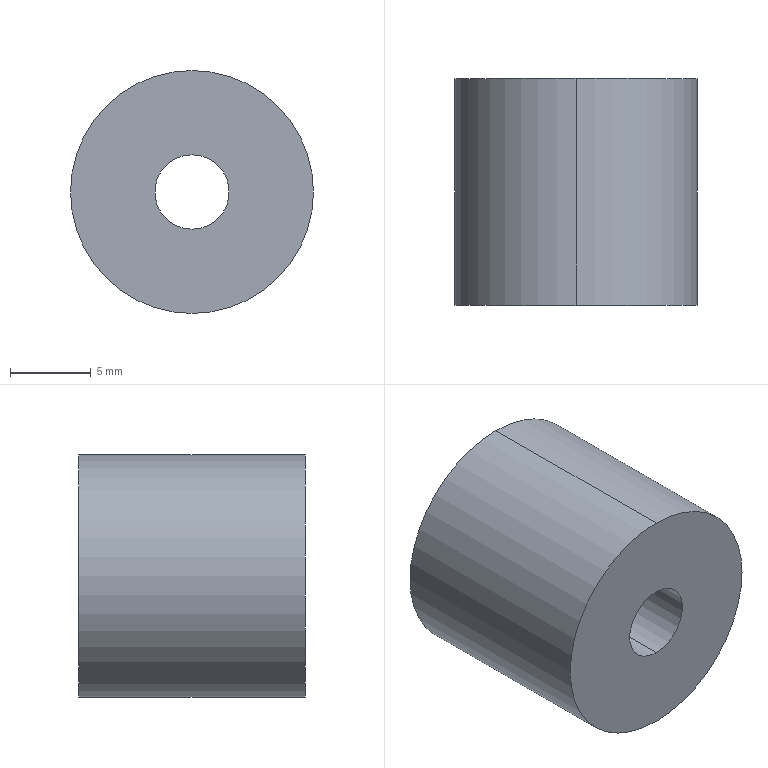Part | STEP file | 1 solid | 9 faces | box 15 x 14 x 15 mm | volume 1932 mm3 | cylinder 6 | plane 3 | commonest cylinder face diameters 4.6 x2 10 x2 15 x2
STEP:
#1=CARTESIAN_POINT('',(0.,0.,0.));
#2=DIRECTION('',(0.,0.,1.));
#3=DIRECTION('',(1.,0.,0.));
#4=AXIS2_PLACEMENT_3D('',#1,#2,#3);
#5=CARTESIAN_POINT('',(0.,14.,7.5));
#6=VERTEX_POINT('',#5);
#7=CARTESIAN_POINT('',(0.,0.,7.5));
#8=VERTEX_POINT('',#7);
#9=CARTESIAN_POINT('',(0.,0.,7.5));
#10=DIRECTION('',(0.,-1.,0.));
#11=VECTOR('',#10,1.);
#12=LINE('',#9,#11);
#13=CARTESIAN_POINT('',(0.,0.,0.));
#14=DIRECTION('',(0.,-1.,0.));
#15=DIRECTION('',(0.,0.,-1.));
#16=AXIS2_PLACEMENT_3D('',#13,#14,#15);
#17=CYLINDRICAL_SURFACE('',#16,7.5);
#18=CARTESIAN_POINT('',(3.142,0.));
#19=DIRECTION('',(0.,1.));
#20=VECTOR('',#19,1.);
#21=LINE('',#18,#20);
#22=(GEOMETRIC_REPRESENTATION_CONTEXT(2)PARAMETRIC_REPRESENTATION_CONTEXT()REPRESENTATION_CONTEXT('',''));
#23=DEFINITIONAL_REPRESENTATION('',(#21),#22);
#24=PCURVE('',#17,#23);
#25=CARTESIAN_POINT('',(0.,0.,0.));
#26=DIRECTION('',(0.,-1.,0.));
#27=DIRECTION('',(0.,0.,-1.));
#28=AXIS2_PLACEMENT_3D('',#25,#26,#27);
#29=CYLINDRICAL_SURFACE('',#28,7.5);
#30=CARTESIAN_POINT('',(3.142,0.));
#31=DIRECTION('',(0.,1.));
#32=VECTOR('',#31,1.);
#33=LINE('',#30,#32);
#34=(GEOMETRIC_REPRESENTATION_CONTEXT(2)PARAMETRIC_REPRESENTATION_CONTEXT()REPRESENTATION_CONTEXT('',''));
#35=DEFINITIONAL_REPRESENTATION('',(#33),#34);
#36=PCURVE('',#29,#35);
#37=SURFACE_CURVE('',#12,(#24,#36),.PCURVE_S1.);
#38=EDGE_CURVE('',#6,#8,#37,.T.);
#39=ORIENTED_EDGE('',*,*,#38,.F.);
#40=CARTESIAN_POINT('',(0.,14.,-7.5));
#41=VERTEX_POINT('',#40);
#42=CARTESIAN_POINT('',(0.,14.,0.));
#43=DIRECTION('',(0.,-1.,0.));
#44=DIRECTION('',(0.,0.,-1.));
#45=AXIS2_PLACEMENT_3D('',#42,#43,#44);
#46=CIRCLE('',#45,7.5);
#47=CARTESIAN_POINT('',(0.,-14.));
#48=DIRECTION('',(1.,0.));
#49=VECTOR('',#48,1.);
#50=LINE('',#47,#49);
#51=(GEOMETRIC_REPRESENTATION_CONTEXT(2)PARAMETRIC_REPRESENTATION_CONTEXT()REPRESENTATION_CONTEXT('',''));
#52=DEFINITIONAL_REPRESENTATION('',(#50),#51);
#53=PCURVE('',#17,#52);
#54=CARTESIAN_POINT('',(-5.,14.,0.));
#55=DIRECTION('',(0.,-1.,0.));
#56=DIRECTION('',(0.,0.,-1.));
#57=AXIS2_PLACEMENT_3D('',#54,#55,#56);
#58=PLANE('',#57);
#59=CARTESIAN_POINT('',(0.,5.));
#60=DIRECTION('',(1.,0.));
#61=AXIS2_PLACEMENT_2D('',#59,#60);
#62=CIRCLE('',#61,7.5);
#63=(GEOMETRIC_REPRESENTATION_CONTEXT(2)PARAMETRIC_REPRESENTATION_CONTEXT()REPRESENTATION_CONTEXT('',''));
#64=DEFINITIONAL_REPRESENTATION('',(#62),#63);
#65=PCURVE('',#58,#64);
#66=SURFACE_CURVE('',#46,(#53,#65),.PCURVE_S1.);
#67=EDGE_CURVE('',#6,#41,#66,.T.);
#68=ORIENTED_EDGE('',*,*,#67,.T.);
#69=CARTESIAN_POINT('',(0.,0.,-7.5));
#70=VERTEX_POINT('',#69);
#71=CARTESIAN_POINT('',(0.,0.,-7.5));
#72=DIRECTION('',(0.,-1.,0.));
#73=VECTOR('',#72,1.);
#74=LINE('',#71,#73);
#75=CARTESIAN_POINT('',(6.283,0.));
#76=DIRECTION('',(0.,1.));
#77=VECTOR('',#76,1.);
#78=LINE('',#75,#77);
#79=(GEOMETRIC_REPRESENTATION_CONTEXT(2)PARAMETRIC_REPRESENTATION_CONTEXT()REPRESENTATION_CONTEXT('',''));
#80=DEFINITIONAL_REPRESENTATION('',(#78),#79);
#81=PCURVE('',#17,#80);
#82=CARTESIAN_POINT('',(0.,0.));
#83=DIRECTION('',(0.,1.));
#84=VECTOR('',#83,1.);
#85=LINE('',#82,#84);
#86=(GEOMETRIC_REPRESENTATION_CONTEXT(2)PARAMETRIC_REPRESENTATION_CONTEXT()REPRESENTATION_CONTEXT('',''));
#87=DEFINITIONAL_REPRESENTATION('',(#85),#86);
#88=PCURVE('',#29,#87);
#89=SURFACE_CURVE('',#74,(#81,#88),.PCURVE_S1.);
#90=EDGE_CURVE('',#41,#70,#89,.T.);
#91=ORIENTED_EDGE('',*,*,#90,.T.);
#92=CARTESIAN_POINT('',(0.,0.,0.));
#93=DIRECTION('',(0.,-1.,0.));
#94=DIRECTION('',(0.,0.,-1.));
#95=AXIS2_PLACEMENT_3D('',#92,#93,#94);
#96=CIRCLE('',#95,7.5);
#97=CARTESIAN_POINT('',(0.,0.));
#98=DIRECTION('',(1.,0.));
#99=VECTOR('',#98,1.);
#100=LINE('',#97,#99);
#101=(GEOMETRIC_REPRESENTATION_CONTEXT(2)PARAMETRIC_REPRESENTATION_CONTEXT()REPRESENTATION_CONTEXT('',''));
#102=DEFINITIONAL_REPRESENTATION('',(#100),#101);
#103=PCURVE('',#17,#102);
#104=CARTESIAN_POINT('',(-7.5,0.,0.));
#105=DIRECTION('',(0.,1.,0.));
#106=DIRECTION('',(0.,0.,1.));
#107=AXIS2_PLACEMENT_3D('',#104,#105,#106);
#108=PLANE('',#107);
#109=CARTESIAN_POINT('',(-7.5,7.5));
#110=CARTESIAN_POINT('',(-7.5,20.49));
#111=CARTESIAN_POINT('',(3.75,13.995));
#112=CARTESIAN_POINT('',(15.,7.5));
#113=CARTESIAN_POINT('',(3.75,1.005));
#114=CARTESIAN_POINT('',(-7.5,-5.49));
#115=CARTESIAN_POINT('',(-7.5,7.5));
#116=(BOUNDED_CURVE()B_SPLINE_CURVE(2,(#109,#110,#111,#112,#113,#114,#115),.UNSPECIFIED.,.T.,.F.)B_SPLINE_CURVE_WITH_KNOTS((1,2,2,2,2,1),(-2.094,0.,2.094,4.189,6.283,8.378),.UNSPECIFIED.)CURVE()GEOMETRIC_REPRESENTATION_ITEM()RATIONAL_B_SPLINE_CURVE((1.,0.5,1.,0.5,1.,0.5,1.))REPRESENTATION_ITEM(''));
#117=(GEOMETRIC_REPRESENTATION_CONTEXT(2)PARAMETRIC_REPRESENTATION_CONTEXT()REPRESENTATION_CONTEXT('',''));
#118=DEFINITIONAL_REPRESENTATION('',(#116),#117);
#119=PCURVE('',#108,#118);
#120=SURFACE_CURVE('',#96,(#103,#119),.PCURVE_S1.);
#121=EDGE_CURVE('',#8,#70,#120,.T.);
#122=ORIENTED_EDGE('',*,*,#121,.F.);
#123=EDGE_LOOP('',(#39,#68,#91,#122));
#124=FACE_BOUND('',#123,.T.);
#125=ADVANCED_FACE('',(#124),#17,.T.);
#126=CARTESIAN_POINT('',(0.,14.,-5.));
#127=VERTEX_POINT('',#126);
#128=CARTESIAN_POINT('',(0.,14.,5.));
#129=VERTEX_POINT('',#128);
#130=CARTESIAN_POINT('',(0.,14.,0.));
#131=DIRECTION('',(0.,-1.,0.));
#132=DIRECTION('',(0.,0.,-1.));
#133=AXIS2_PLACEMENT_3D('',#130,#131,#132);
#134=CIRCLE('',#133,5.);
#135=CARTESIAN_POINT('',(0.,5.));
#136=DIRECTION('',(1.,0.));
#137=AXIS2_PLACEMENT_2D('',#135,#136);
#138=CIRCLE('',#137,5.);
#139=(GEOMETRIC_REPRESENTATION_CONTEXT(2)PARAMETRIC_REPRESENTATION_CONTEXT()REPRESENTATION_CONTEXT('',''));
#140=DEFINITIONAL_REPRESENTATION('',(#138),#139);
#141=PCURVE('',#58,#140);
#142=CARTESIAN_POINT('',(0.,0.,0.));
#143=DIRECTION('',(0.,-1.,0.));
#144=DIRECTION('',(0.,0.,-1.));
#145=AXIS2_PLACEMENT_3D('',#142,#143,#144);
#146=CYLINDRICAL_SURFACE('',#145,5.);
#147=CARTESIAN_POINT('',(0.,-14.));
#148=DIRECTION('',(1.,0.));
#149=VECTOR('',#148,1.);
#150=LINE('',#147,#149);
#151=(GEOMETRIC_REPRESENTATION_CONTEXT(2)PARAMETRIC_REPRESENTATION_CONTEXT()REPRESENTATION_CONTEXT('',''));
#152=DEFINITIONAL_REPRESENTATION('',(#150),#151);
#153=PCURVE('',#146,#152);
#154=SURFACE_CURVE('',#134,(#141,#153),.PCURVE_S1.);
#155=EDGE_CURVE('',#127,#129,#154,.T.);
#156=ORIENTED_EDGE('',*,*,#155,.T.);
#157=CARTESIAN_POINT('',(0.,14.,0.));
#158=DIRECTION('',(0.,-1.,0.));
#159=DIRECTION('',(0.,0.,-1.));
#160=AXIS2_PLACEMENT_3D('',#157,#158,#159);
#161=CIRCLE('',#160,5.);
#162=CARTESIAN_POINT('',(0.,5.));
#163=DIRECTION('',(1.,0.));
#164=AXIS2_PLACEMENT_2D('',#162,#163);
#165=CIRCLE('',#164,5.);
#166=(GEOMETRIC_REPRESENTATION_CONTEXT(2)PARAMETRIC_REPRESENTATION_CONTEXT()REPRESENTATION_CONTEXT('',''));
#167=DEFINITIONAL_REPRESENTATION('',(#165),#166);
#168=PCURVE('',#58,#167);
#169=CARTESIAN_POINT('',(0.,0.,0.));
#170=DIRECTION('',(0.,-1.,0.));
#171=DIRECTION('',(0.,0.,-1.));
#172=AXIS2_PLACEMENT_3D('',#169,#170,#171);
#173=CYLINDRICAL_SURFACE('',#172,5.);
#174=CARTESIAN_POINT('',(0.,-14.));
#175=DIRECTION('',(1.,0.));
#176=VECTOR('',#175,1.);
#177=LINE('',#174,#176);
#178=(GEOMETRIC_REPRESENTATION_CONTEXT(2)PARAMETRIC_REPRESENTATION_CONTEXT()REPRESENTATION_CONTEXT('',''));
#179=DEFINITIONAL_REPRESENTATION('',(#177),#178);
#180=PCURVE('',#173,#179);
#181=SURFACE_CURVE('',#161,(#168,#180),.PCURVE_S1.);
#182=EDGE_CURVE('',#129,#127,#181,.T.);
#183=ORIENTED_EDGE('',*,*,#182,.T.);
#184=EDGE_LOOP('',(#156,#183));
#185=FACE_BOUND('',#184,.T.);
#186=CARTESIAN_POINT('',(0.,14.,0.));
#187=DIRECTION('',(0.,-1.,0.));
#188=DIRECTION('',(0.,0.,-1.));
#189=AXIS2_PLACEMENT_3D('',#186,#187,#188);
#190=CIRCLE('',#189,7.5);
#191=CARTESIAN_POINT('',(0.,5.));
#192=DIRECTION('',(1.,0.));
#193=AXIS2_PLACEMENT_2D('',#191,#192);
#194=CIRCLE('',#193,7.5);
#195=(GEOMETRIC_REPRESENTATION_CONTEXT(2)PARAMETRIC_REPRESENTATION_CONTEXT()REPRESENTATION_CONTEXT('',''));
#196=DEFINITIONAL_REPRESENTATION('',(#194),#195);
#197=PCURVE('',#58,#196);
#198=CARTESIAN_POINT('',(0.,-14.));
#199=DIRECTION('',(1.,0.));
#200=VECTOR('',#199,1.);
#201=LINE('',#198,#200);
#202=(GEOMETRIC_REPRESENTATION_CONTEXT(2)PARAMETRIC_REPRESENTATION_CONTEXT()REPRESENTATION_CONTEXT('',''));
#203=DEFINITIONAL_REPRESENTATION('',(#201),#202);
#204=PCURVE('',#29,#203);
#205=SURFACE_CURVE('',#190,(#197,#204),.PCURVE_S1.);
#206=EDGE_CURVE('',#41,#6,#205,.T.);
#207=ORIENTED_EDGE('',*,*,#206,.F.);
#208=ORIENTED_EDGE('',*,*,#67,.F.);
#209=EDGE_LOOP('',(#207,#208));
#210=FACE_BOUND('',#209,.T.);
#211=ADVANCED_FACE('',(#185,#210),#58,.F.);
#212=CARTESIAN_POINT('',(0.,9.,-5.));
#213=VERTEX_POINT('',#212);
#214=CARTESIAN_POINT('',(0.,9.,5.));
#215=VERTEX_POINT('',#214);
#216=CARTESIAN_POINT('',(0.,9.,0.));
#217=DIRECTION('',(0.,-1.,0.));
#218=DIRECTION('',(0.,0.,-1.));
#219=AXIS2_PLACEMENT_3D('',#216,#217,#218);
#220=CIRCLE('',#219,5.);
#221=CARTESIAN_POINT('',(0.,-9.));
#222=DIRECTION('',(1.,0.));
#223=VECTOR('',#222,1.);
#224=LINE('',#221,#223);
#225=(GEOMETRIC_REPRESENTATION_CONTEXT(2)PARAMETRIC_REPRESENTATION_CONTEXT()REPRESENTATION_CONTEXT('',''));
#226=DEFINITIONAL_REPRESENTATION('',(#224),#225);
#227=PCURVE('',#146,#226);
#228=CARTESIAN_POINT('',(-2.3,9.,0.));
#229=DIRECTION('',(0.,-1.,0.));
#230=DIRECTION('',(0.,0.,-1.));
#231=AXIS2_PLACEMENT_3D('',#228,#229,#230);
#232=PLANE('',#231);
#233=CARTESIAN_POINT('',(0.,2.3));
#234=DIRECTION('',(1.,0.));
#235=AXIS2_PLACEMENT_2D('',#233,#234);
#236=CIRCLE('',#235,5.);
#237=(GEOMETRIC_REPRESENTATION_CONTEXT(2)PARAMETRIC_REPRESENTATION_CONTEXT()REPRESENTATION_CONTEXT('',''));
#238=DEFINITIONAL_REPRESENTATION('',(#236),#237);
#239=PCURVE('',#232,#238);
#240=SURFACE_CURVE('',#220,(#227,#239),.PCURVE_S1.);
#241=EDGE_CURVE('',#213,#215,#240,.T.);
#242=ORIENTED_EDGE('',*,*,#241,.F.);
#243=CARTESIAN_POINT('',(0.,0.,-5.));
#244=DIRECTION('',(0.,-1.,0.));
#245=VECTOR('',#244,1.);
#246=LINE('',#243,#245);
#247=CARTESIAN_POINT('',(0.,0.));
#248=DIRECTION('',(0.,1.));
#249=VECTOR('',#248,1.);
#250=LINE('',#247,#249);
#251=(GEOMETRIC_REPRESENTATION_CONTEXT(2)PARAMETRIC_REPRESENTATION_CONTEXT()REPRESENTATION_CONTEXT('',''));
#252=DEFINITIONAL_REPRESENTATION('',(#250),#251);
#253=PCURVE('',#146,#252);
#254=CARTESIAN_POINT('',(6.283,0.));
#255=DIRECTION('',(0.,1.));
#256=VECTOR('',#255,1.);
#257=LINE('',#254,#256);
#258=(GEOMETRIC_REPRESENTATION_CONTEXT(2)PARAMETRIC_REPRESENTATION_CONTEXT()REPRESENTATION_CONTEXT('',''));
#259=DEFINITIONAL_REPRESENTATION('',(#257),#258);
#260=PCURVE('',#173,#259);
#261=SURFACE_CURVE('',#246,(#253,#260),.PCURVE_S1.);
#262=EDGE_CURVE('',#127,#213,#261,.T.);
#263=ORIENTED_EDGE('',*,*,#262,.F.);
#264=ORIENTED_EDGE('',*,*,#155,.T.);
#265=CARTESIAN_POINT('',(0.,0.,5.));
#266=DIRECTION('',(0.,-1.,0.));
#267=VECTOR('',#266,1.);
#268=LINE('',#265,#267);
#269=CARTESIAN_POINT('',(3.142,0.));
#270=DIRECTION('',(0.,1.));
#271=VECTOR('',#270,1.);
#272=LINE('',#269,#271);
#273=(GEOMETRIC_REPRESENTATION_CONTEXT(2)PARAMETRIC_REPRESENTATION_CONTEXT()REPRESENTATION_CONTEXT('',''));
#274=DEFINITIONAL_REPRESENTATION('',(#272),#273);
#275=PCURVE('',#146,#274);
#276=CARTESIAN_POINT('',(3.142,0.));
#277=DIRECTION('',(0.,1.));
#278=VECTOR('',#277,1.);
#279=LINE('',#276,#278);
#280=(GEOMETRIC_REPRESENTATION_CONTEXT(2)PARAMETRIC_REPRESENTATION_CONTEXT()REPRESENTATION_CONTEXT('',''));
#281=DEFINITIONAL_REPRESENTATION('',(#279),#280);
#282=PCURVE('',#173,#281);
#283=SURFACE_CURVE('',#268,(#275,#282),.PCURVE_S1.);
#284=EDGE_CURVE('',#129,#215,#283,.T.);
#285=ORIENTED_EDGE('',*,*,#284,.T.);
#286=EDGE_LOOP('',(#242,#263,#264,#285));
#287=FACE_BOUND('',#286,.F.);
#288=ADVANCED_FACE('',(#287),#146,.F.);
#289=CARTESIAN_POINT('',(0.,9.,-2.3));
#290=VERTEX_POINT('',#289);
#291=CARTESIAN_POINT('',(0.,9.,2.3));
#292=VERTEX_POINT('',#291);
#293=CARTESIAN_POINT('',(0.,9.,0.));
#294=DIRECTION('',(0.,-1.,0.));
#295=DIRECTION('',(0.,0.,-1.));
#296=AXIS2_PLACEMENT_3D('',#293,#294,#295);
#297=CIRCLE('',#296,2.3);
#298=CARTESIAN_POINT('',(0.,2.3));
#299=DIRECTION('',(1.,0.));
#300=AXIS2_PLACEMENT_2D('',#298,#299);
#301=CIRCLE('',#300,2.3);
#302=(GEOMETRIC_REPRESENTATION_CONTEXT(2)PARAMETRIC_REPRESENTATION_CONTEXT()REPRESENTATION_CONTEXT('',''));
#303=DEFINITIONAL_REPRESENTATION('',(#301),#302);
#304=PCURVE('',#232,#303);
#305=CARTESIAN_POINT('',(0.,0.,0.));
#306=DIRECTION('',(0.,-1.,0.));
#307=DIRECTION('',(0.,0.,-1.));
#308=AXIS2_PLACEMENT_3D('',#305,#306,#307);
#309=CYLINDRICAL_SURFACE('',#308,2.3);
#310=CARTESIAN_POINT('',(0.,-9.));
#311=DIRECTION('',(1.,0.));
#312=VECTOR('',#311,1.);
#313=LINE('',#310,#312);
#314=(GEOMETRIC_REPRESENTATION_CONTEXT(2)PARAMETRIC_REPRESENTATION_CONTEXT()REPRESENTATION_CONTEXT('',''));
#315=DEFINITIONAL_REPRESENTATION('',(#313),#314);
#316=PCURVE('',#309,#315);
#317=SURFACE_CURVE('',#297,(#304,#316),.PCURVE_S1.);
#318=EDGE_CURVE('',#290,#292,#317,.T.);
#319=ORIENTED_EDGE('',*,*,#318,.T.);
#320=CARTESIAN_POINT('',(0.,9.,0.));
#321=DIRECTION('',(0.,-1.,0.));
#322=DIRECTION('',(0.,0.,-1.));
#323=AXIS2_PLACEMENT_3D('',#320,#321,#322);
#324=CIRCLE('',#323,2.3);
#325=CARTESIAN_POINT('',(0.,2.3));
#326=DIRECTION('',(1.,0.));
#327=AXIS2_PLACEMENT_2D('',#325,#326);
#328=CIRCLE('',#327,2.3);
#329=(GEOMETRIC_REPRESENTATION_CONTEXT(2)PARAMETRIC_REPRESENTATION_CONTEXT()REPRESENTATION_CONTEXT('',''));
#330=DEFINITIONAL_REPRESENTATION('',(#328),#329);
#331=PCURVE('',#232,#330);
#332=CARTESIAN_POINT('',(0.,0.,0.));
#333=DIRECTION('',(0.,-1.,0.));
#334=DIRECTION('',(0.,0.,-1.));
#335=AXIS2_PLACEMENT_3D('',#332,#333,#334);
#336=CYLINDRICAL_SURFACE('',#335,2.3);
#337=CARTESIAN_POINT('',(0.,-9.));
#338=DIRECTION('',(1.,0.));
#339=VECTOR('',#338,1.);
#340=LINE('',#337,#339);
#341=(GEOMETRIC_REPRESENTATION_CONTEXT(2)PARAMETRIC_REPRESENTATION_CONTEXT()REPRESENTATION_CONTEXT('',''));
#342=DEFINITIONAL_REPRESENTATION('',(#340),#341);
#343=PCURVE('',#336,#342);
#344=SURFACE_CURVE('',#324,(#331,#343),.PCURVE_S1.);
#345=EDGE_CURVE('',#292,#290,#344,.T.);
#346=ORIENTED_EDGE('',*,*,#345,.T.);
#347=EDGE_LOOP('',(#319,#346));
#348=FACE_BOUND('',#347,.T.);
#349=ORIENTED_EDGE('',*,*,#241,.F.);
#350=CARTESIAN_POINT('',(0.,9.,0.));
#351=DIRECTION('',(0.,-1.,0.));
#352=DIRECTION('',(0.,0.,-1.));
#353=AXIS2_PLACEMENT_3D('',#350,#351,#352);
#354=CIRCLE('',#353,5.);
#355=CARTESIAN_POINT('',(0.,2.3));
#356=DIRECTION('',(1.,0.));
#357=AXIS2_PLACEMENT_2D('',#355,#356);
#358=CIRCLE('',#357,5.);
#359=(GEOMETRIC_REPRESENTATION_CONTEXT(2)PARAMETRIC_REPRESENTATION_CONTEXT()REPRESENTATION_CONTEXT('',''));
#360=DEFINITIONAL_REPRESENTATION('',(#358),#359);
#361=PCURVE('',#232,#360);
#362=CARTESIAN_POINT('',(0.,-9.));
#363=DIRECTION('',(1.,0.));
#364=VECTOR('',#363,1.);
#365=LINE('',#362,#364);
#366=(GEOMETRIC_REPRESENTATION_CONTEXT(2)PARAMETRIC_REPRESENTATION_CONTEXT()REPRESENTATION_CONTEXT('',''));
#367=DEFINITIONAL_REPRESENTATION('',(#365),#366);
#368=PCURVE('',#173,#367);
#369=SURFACE_CURVE('',#354,(#361,#368),.PCURVE_S1.);
#370=EDGE_CURVE('',#215,#213,#369,.T.);
#371=ORIENTED_EDGE('',*,*,#370,.F.);
#372=EDGE_LOOP('',(#349,#371));
#373=FACE_BOUND('',#372,.T.);
#374=ADVANCED_FACE('',(#348,#373),#232,.F.);
#375=CARTESIAN_POINT('',(0.,0.,-2.3));
#376=VERTEX_POINT('',#375);
#377=CARTESIAN_POINT('',(0.,0.,2.3));
#378=VERTEX_POINT('',#377);
#379=CARTESIAN_POINT('',(0.,0.,0.));
#380=DIRECTION('',(0.,-1.,0.));
#381=DIRECTION('',(0.,0.,-1.));
#382=AXIS2_PLACEMENT_3D('',#379,#380,#381);
#383=CIRCLE('',#382,2.3);
#384=CARTESIAN_POINT('',(0.,0.));
#385=DIRECTION('',(1.,0.));
#386=VECTOR('',#385,1.);
#387=LINE('',#384,#386);
#388=(GEOMETRIC_REPRESENTATION_CONTEXT(2)PARAMETRIC_REPRESENTATION_CONTEXT()REPRESENTATION_CONTEXT('',''));
#389=DEFINITIONAL_REPRESENTATION('',(#387),#388);
#390=PCURVE('',#309,#389);
#391=CARTESIAN_POINT('',(-2.3,7.5));
#392=CARTESIAN_POINT('',(-2.3,11.484));
#393=CARTESIAN_POINT('',(1.15,9.492));
#394=CARTESIAN_POINT('',(4.6,7.5));
#395=CARTESIAN_POINT('',(1.15,5.508));
#396=CARTESIAN_POINT('',(-2.3,3.516));
#397=CARTESIAN_POINT('',(-2.3,7.5));
#398=(BOUNDED_CURVE()B_SPLINE_CURVE(2,(#391,#392,#393,#394,#395,#396,#397),.UNSPECIFIED.,.T.,.F.)B_SPLINE_CURVE_WITH_KNOTS((1,2,2,2,2,1),(-2.094,0.,2.094,4.189,6.283,8.378),.UNSPECIFIED.)CURVE()GEOMETRIC_REPRESENTATION_ITEM()RATIONAL_B_SPLINE_CURVE((1.,0.5,1.,0.5,1.,0.5,1.))REPRESENTATION_ITEM(''));
#399=(GEOMETRIC_REPRESENTATION_CONTEXT(2)PARAMETRIC_REPRESENTATION_CONTEXT()REPRESENTATION_CONTEXT('',''));
#400=DEFINITIONAL_REPRESENTATION('',(#398),#399);
#401=PCURVE('',#108,#400);
#402=SURFACE_CURVE('',#383,(#390,#401),.PCURVE_S1.);
#403=EDGE_CURVE('',#376,#378,#402,.T.);
#404=ORIENTED_EDGE('',*,*,#403,.F.);
#405=CARTESIAN_POINT('',(0.,0.,-2.3));
#406=DIRECTION('',(0.,-1.,0.));
#407=VECTOR('',#406,1.);
#408=LINE('',#405,#407);
#409=CARTESIAN_POINT('',(0.,0.));
#410=DIRECTION('',(0.,1.));
#411=VECTOR('',#410,1.);
#412=LINE('',#409,#411);
#413=(GEOMETRIC_REPRESENTATION_CONTEXT(2)PARAMETRIC_REPRESENTATION_CONTEXT()REPRESENTATION_CONTEXT('',''));
#414=DEFINITIONAL_REPRESENTATION('',(#412),#413);
#415=PCURVE('',#309,#414);
#416=CARTESIAN_POINT('',(6.283,0.));
#417=DIRECTION('',(0.,1.));
#418=VECTOR('',#417,1.);
#419=LINE('',#416,#418);
#420=(GEOMETRIC_REPRESENTATION_CONTEXT(2)PARAMETRIC_REPRESENTATION_CONTEXT()REPRESENTATION_CONTEXT('',''));
#421=DEFINITIONAL_REPRESENTATION('',(#419),#420);
#422=PCURVE('',#336,#421);
#423=SURFACE_CURVE('',#408,(#415,#422),.PCURVE_S1.);
#424=EDGE_CURVE('',#290,#376,#423,.T.);
#425=ORIENTED_EDGE('',*,*,#424,.F.);
#426=ORIENTED_EDGE('',*,*,#318,.T.);
#427=CARTESIAN_POINT('',(0.,0.,2.3));
#428=DIRECTION('',(0.,-1.,0.));
#429=VECTOR('',#428,1.);
#430=LINE('',#427,#429);
#431=CARTESIAN_POINT('',(3.142,0.));
#432=DIRECTION('',(0.,1.));
#433=VECTOR('',#432,1.);
#434=LINE('',#431,#433);
#435=(GEOMETRIC_REPRESENTATION_CONTEXT(2)PARAMETRIC_REPRESENTATION_CONTEXT()REPRESENTATION_CONTEXT('',''));
#436=DEFINITIONAL_REPRESENTATION('',(#434),#435);
#437=PCURVE('',#309,#436);
#438=CARTESIAN_POINT('',(3.142,0.));
#439=DIRECTION('',(0.,1.));
#440=VECTOR('',#439,1.);
#441=LINE('',#438,#440);
#442=(GEOMETRIC_REPRESENTATION_CONTEXT(2)PARAMETRIC_REPRESENTATION_CONTEXT()REPRESENTATION_CONTEXT('',''));
#443=DEFINITIONAL_REPRESENTATION('',(#441),#442);
#444=PCURVE('',#336,#443);
#445=SURFACE_CURVE('',#430,(#437,#444),.PCURVE_S1.);
#446=EDGE_CURVE('',#292,#378,#445,.T.);
#447=ORIENTED_EDGE('',*,*,#446,.T.);
#448=EDGE_LOOP('',(#404,#425,#426,#447));
#449=FACE_BOUND('',#448,.F.);
#450=ADVANCED_FACE('',(#449),#309,.F.);
#451=CARTESIAN_POINT('',(0.,0.,0.));
#452=DIRECTION('',(0.,-1.,0.));
#453=DIRECTION('',(0.,0.,-1.));
#454=AXIS2_PLACEMENT_3D('',#451,#452,#453);
#455=CIRCLE('',#454,7.5);
#456=CARTESIAN_POINT('',(-7.5,7.5));
#457=CARTESIAN_POINT('',(-7.5,20.49));
#458=CARTESIAN_POINT('',(3.75,13.995));
#459=CARTESIAN_POINT('',(15.,7.5));
#460=CARTESIAN_POINT('',(3.75,1.005));
#461=CARTESIAN_POINT('',(-7.5,-5.49));
#462=CARTESIAN_POINT('',(-7.5,7.5));
#463=(BOUNDED_CURVE()B_SPLINE_CURVE(2,(#456,#457,#458,#459,#460,#461,#462),.UNSPECIFIED.,.T.,.F.)B_SPLINE_CURVE_WITH_KNOTS((1,2,2,2,2,1),(-2.094,0.,2.094,4.189,6.283,8.378),.UNSPECIFIED.)CURVE()GEOMETRIC_REPRESENTATION_ITEM()RATIONAL_B_SPLINE_CURVE((1.,0.5,1.,0.5,1.,0.5,1.))REPRESENTATION_ITEM(''));
#464=(GEOMETRIC_REPRESENTATION_CONTEXT(2)PARAMETRIC_REPRESENTATION_CONTEXT()REPRESENTATION_CONTEXT('',''));
#465=DEFINITIONAL_REPRESENTATION('',(#463),#464);
#466=PCURVE('',#108,#465);
#467=CARTESIAN_POINT('',(0.,0.));
#468=DIRECTION('',(1.,0.));
#469=VECTOR('',#468,1.);
#470=LINE('',#467,#469);
#471=(GEOMETRIC_REPRESENTATION_CONTEXT(2)PARAMETRIC_REPRESENTATION_CONTEXT()REPRESENTATION_CONTEXT('',''));
#472=DEFINITIONAL_REPRESENTATION('',(#470),#471);
#473=PCURVE('',#29,#472);
#474=SURFACE_CURVE('',#455,(#466,#473),.PCURVE_S1.);
#475=EDGE_CURVE('',#70,#8,#474,.T.);
#476=ORIENTED_EDGE('',*,*,#475,.T.);
#477=ORIENTED_EDGE('',*,*,#121,.T.);
#478=EDGE_LOOP('',(#476,#477));
#479=FACE_BOUND('',#478,.T.);
#480=ORIENTED_EDGE('',*,*,#403,.F.);
#481=CARTESIAN_POINT('',(0.,0.,0.));
#482=DIRECTION('',(0.,-1.,0.));
#483=DIRECTION('',(0.,0.,-1.));
#484=AXIS2_PLACEMENT_3D('',#481,#482,#483);
#485=CIRCLE('',#484,2.3);
#486=CARTESIAN_POINT('',(-2.3,7.5));
#487=CARTESIAN_POINT('',(-2.3,11.484));
#488=CARTESIAN_POINT('',(1.15,9.492));
#489=CARTESIAN_POINT('',(4.6,7.5));
#490=CARTESIAN_POINT('',(1.15,5.508));
#491=CARTESIAN_POINT('',(-2.3,3.516));
#492=CARTESIAN_POINT('',(-2.3,7.5));
#493=(BOUNDED_CURVE()B_SPLINE_CURVE(2,(#486,#487,#488,#489,#490,#491,#492),.UNSPECIFIED.,.T.,.F.)B_SPLINE_CURVE_WITH_KNOTS((1,2,2,2,2,1),(-2.094,0.,2.094,4.189,6.283,8.378),.UNSPECIFIED.)CURVE()GEOMETRIC_REPRESENTATION_ITEM()RATIONAL_B_SPLINE_CURVE((1.,0.5,1.,0.5,1.,0.5,1.))REPRESENTATION_ITEM(''));
#494=(GEOMETRIC_REPRESENTATION_CONTEXT(2)PARAMETRIC_REPRESENTATION_CONTEXT()REPRESENTATION_CONTEXT('',''));
#495=DEFINITIONAL_REPRESENTATION('',(#493),#494);
#496=PCURVE('',#108,#495);
#497=CARTESIAN_POINT('',(0.,0.));
#498=DIRECTION('',(1.,0.));
#499=VECTOR('',#498,1.);
#500=LINE('',#497,#499);
#501=(GEOMETRIC_REPRESENTATION_CONTEXT(2)PARAMETRIC_REPRESENTATION_CONTEXT()REPRESENTATION_CONTEXT('',''));
#502=DEFINITIONAL_REPRESENTATION('',(#500),#501);
#503=PCURVE('',#336,#502);
#504=SURFACE_CURVE('',#485,(#496,#503),.PCURVE_S1.);
#505=EDGE_CURVE('',#378,#376,#504,.T.);
#506=ORIENTED_EDGE('',*,*,#505,.F.);
#507=EDGE_LOOP('',(#480,#506));
#508=FACE_BOUND('',#507,.T.);
#509=ADVANCED_FACE('',(#479,#508),#108,.F.);
#510=ORIENTED_EDGE('',*,*,#424,.T.);
#511=ORIENTED_EDGE('',*,*,#505,.F.);
#512=ORIENTED_EDGE('',*,*,#446,.F.);
#513=ORIENTED_EDGE('',*,*,#345,.T.);
#514=EDGE_LOOP('',(#510,#511,#512,#513));
#515=FACE_BOUND('',#514,.F.);
#516=ADVANCED_FACE('',(#515),#336,.F.);
#517=ORIENTED_EDGE('',*,*,#262,.T.);
#518=ORIENTED_EDGE('',*,*,#370,.F.);
#519=ORIENTED_EDGE('',*,*,#284,.F.);
#520=ORIENTED_EDGE('',*,*,#182,.T.);
#521=EDGE_LOOP('',(#517,#518,#519,#520));
#522=FACE_BOUND('',#521,.F.);
#523=ADVANCED_FACE('',(#522),#173,.F.);
#524=ORIENTED_EDGE('',*,*,#206,.T.);
#525=ORIENTED_EDGE('',*,*,#38,.T.);
#526=ORIENTED_EDGE('',*,*,#475,.F.);
#527=ORIENTED_EDGE('',*,*,#90,.F.);
#528=EDGE_LOOP('',(#524,#525,#526,#527));
#529=FACE_BOUND('',#528,.T.);
#530=ADVANCED_FACE('',(#529),#29,.T.);
#531=CLOSED_SHELL('',(#125,#211,#288,#374,#450,#509,#516,#523,#530));
#532=MANIFOLD_SOLID_BREP('',#531);
#533=(LENGTH_UNIT()NAMED_UNIT(*)SI_UNIT(.MILLI.,.METRE.));
#534=UNCERTAINTY_MEASURE_WITH_UNIT(LENGTH_MEASURE(0.0000001),#533,'','');
#535=(NAMED_UNIT(*)PLANE_ANGLE_UNIT()SI_UNIT($,.RADIAN.));
#536=(NAMED_UNIT(*)SI_UNIT($,.STERADIAN.)SOLID_ANGLE_UNIT());
#537=(GEOMETRIC_REPRESENTATION_CONTEXT(3)GLOBAL_UNCERTAINTY_ASSIGNED_CONTEXT((#534))GLOBAL_UNIT_ASSIGNED_CONTEXT((#533,#535,#536))REPRESENTATION_CONTEXT('',''));
#538=ADVANCED_BREP_SHAPE_REPRESENTATION('',(#4,#532),#537);